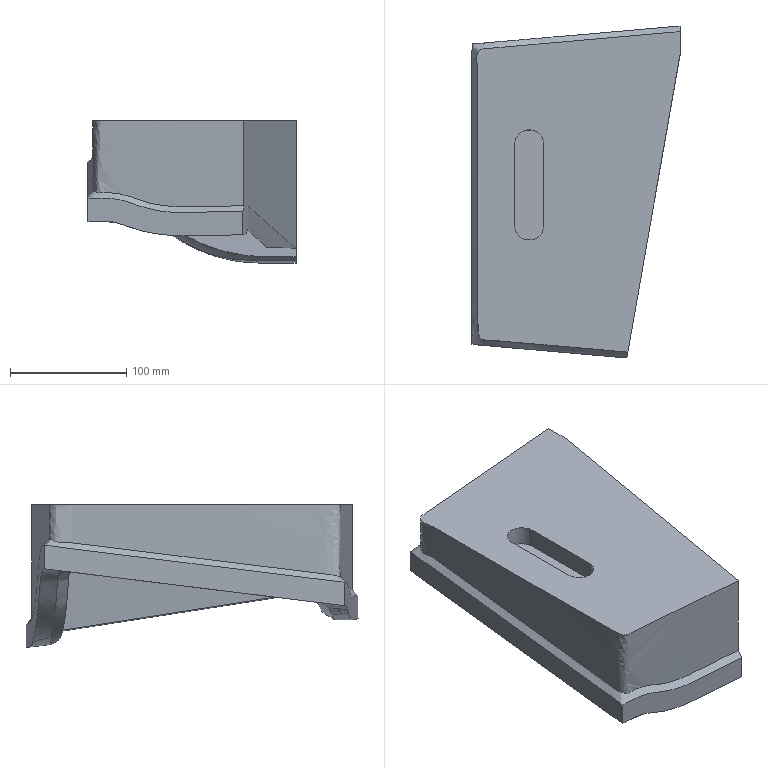Part | NX | features solid 2 | 1 solid | 46 faces | box 179.349 x 286.186 x 123.111 mm | volume 2159734 mm3 | spline 20 | plane 18 | cylinder 8 | commonest cylinder face diameters 30 x6 25 x2